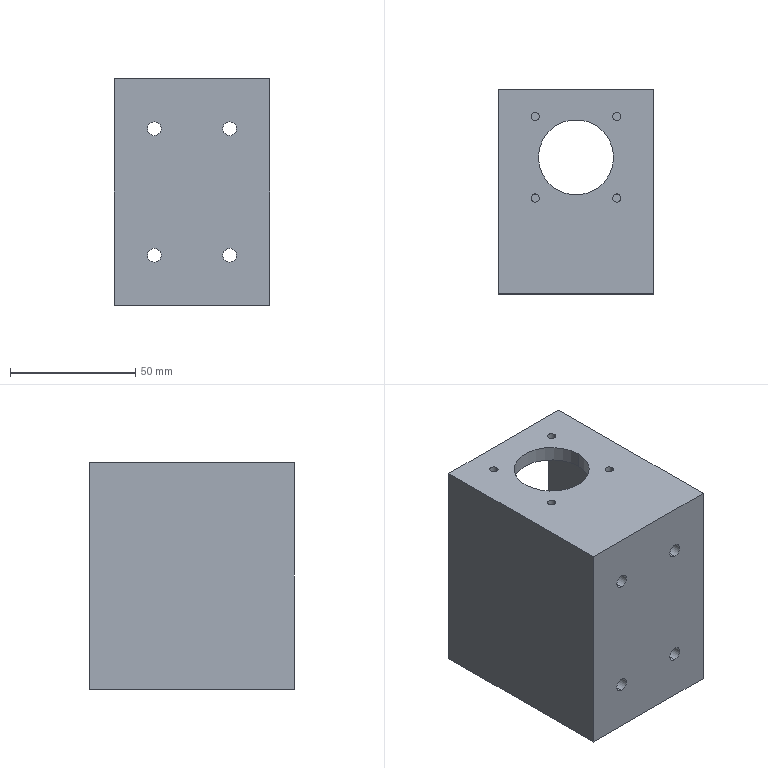Part | Creo | features CURVE 7, CUT 4, DATUM PLANE 3, PROTRUSION 2, CHAMFER 1, COORDINATE SYSTEM 1 | 1 solid | 45 faces | box 62 x 81.5 x 90.5 mm | volume 211765 mm3 | cylinder 26 | plane 19 | commonest cylinder face diameters 3.3 x8 5.5 x8 4.2 x6 30 x2 34 x2
STEP:
#1=CARTESIAN_POINT('',(0.,0.,0.));
#2=DIRECTION('',(0.,0.,1.));
#3=DIRECTION('',(1.,0.,0.));
#4=AXIS2_PLACEMENT_3D('',#1,#2,#3);
#5=CARTESIAN_POINT('',(31.,27.,0.));
#6=VERTEX_POINT('',#5);
#7=CARTESIAN_POINT('',(-31.,27.,0.));
#8=VERTEX_POINT('',#7);
#9=CARTESIAN_POINT('',(31.,27.,0.));
#10=DIRECTION('',(-1.,0.,0.));
#11=VECTOR('',#10,62.);
#12=LINE('',#9,#11);
#13=EDGE_CURVE('',#6,#8,#12,.T.);
#14=ORIENTED_EDGE('',*,*,#13,.T.);
#15=CARTESIAN_POINT('',(-31.,-54.5,0.));
#16=VERTEX_POINT('',#15);
#17=CARTESIAN_POINT('',(-31.,27.,0.));
#18=DIRECTION('',(0.,-1.,0.));
#19=VECTOR('',#18,81.5);
#20=LINE('',#17,#19);
#21=EDGE_CURVE('',#8,#16,#20,.T.);
#22=ORIENTED_EDGE('',*,*,#21,.T.);
#23=CARTESIAN_POINT('',(31.,-54.5,0.));
#24=VERTEX_POINT('',#23);
#25=CARTESIAN_POINT('',(-31.,-54.5,0.));
#26=DIRECTION('',(1.,0.,0.));
#27=VECTOR('',#26,62.);
#28=LINE('',#25,#27);
#29=EDGE_CURVE('',#16,#24,#28,.T.);
#30=ORIENTED_EDGE('',*,*,#29,.T.);
#31=CARTESIAN_POINT('',(31.,-54.5,0.));
#32=DIRECTION('',(0.,1.,0.));
#33=VECTOR('',#32,81.5);
#34=LINE('',#31,#33);
#35=EDGE_CURVE('',#24,#6,#34,.T.);
#36=ORIENTED_EDGE('',*,*,#35,.T.);
#37=EDGE_LOOP('',(#14,#22,#30,#36));
#38=FACE_OUTER_BOUND('',#37,.F.);
#39=CARTESIAN_POINT('',(0.,-17.,0.));
#40=VERTEX_POINT('',#39);
#41=CARTESIAN_POINT('',(0.,17.,0.));
#42=VERTEX_POINT('',#41);
#43=CARTESIAN_POINT('',(0.,0.,0.));
#44=DIRECTION('',(0.,0.,-1.));
#45=DIRECTION('',(0.,-1.,0.));
#46=AXIS2_PLACEMENT_3D('',#43,#44,#45);
#47=CIRCLE('',#46,17.);
#48=EDGE_CURVE('',#40,#42,#47,.T.);
#49=ORIENTED_EDGE('',*,*,#48,.T.);
#50=CARTESIAN_POINT('',(0.,0.,0.));
#51=DIRECTION('',(0.,0.,-1.));
#52=DIRECTION('',(0.,1.,0.));
#53=AXIS2_PLACEMENT_3D('',#50,#51,#52);
#54=CIRCLE('',#53,17.);
#55=EDGE_CURVE('',#42,#40,#54,.T.);
#56=ORIENTED_EDGE('',*,*,#55,.T.);
#57=EDGE_LOOP('',(#49,#56));
#58=FACE_BOUND('',#57,.F.);
#59=CARTESIAN_POINT('',(0.,18.9,0.));
#60=VERTEX_POINT('',#59);
#61=CARTESIAN_POINT('',(0.,23.1,0.));
#62=VERTEX_POINT('',#61);
#63=CARTESIAN_POINT('',(0.,21.,0.));
#64=DIRECTION('',(0.,0.,-1.));
#65=DIRECTION('',(0.,-1.,0.));
#66=AXIS2_PLACEMENT_3D('',#63,#64,#65);
#67=CIRCLE('',#66,2.1);
#68=EDGE_CURVE('',#60,#62,#67,.T.);
#69=ORIENTED_EDGE('',*,*,#68,.T.);
#70=CARTESIAN_POINT('',(0.,21.,0.));
#71=DIRECTION('',(0.,0.,-1.));
#72=DIRECTION('',(0.,1.,0.));
#73=AXIS2_PLACEMENT_3D('',#70,#71,#72);
#74=CIRCLE('',#73,2.1);
#75=EDGE_CURVE('',#62,#60,#74,.T.);
#76=ORIENTED_EDGE('',*,*,#75,.T.);
#77=EDGE_LOOP('',(#69,#76));
#78=FACE_BOUND('',#77,.F.);
#79=CARTESIAN_POINT('',(-18.187,-12.6,0.));
#80=VERTEX_POINT('',#79);
#81=CARTESIAN_POINT('',(-18.187,-8.4,0.));
#82=VERTEX_POINT('',#81);
#83=CARTESIAN_POINT('',(-18.187,-10.5,0.));
#84=DIRECTION('',(0.,0.,-1.));
#85=DIRECTION('',(0.,-1.,0.));
#86=AXIS2_PLACEMENT_3D('',#83,#84,#85);
#87=CIRCLE('',#86,2.1);
#88=EDGE_CURVE('',#80,#82,#87,.T.);
#89=ORIENTED_EDGE('',*,*,#88,.T.);
#90=CARTESIAN_POINT('',(-18.187,-10.5,0.));
#91=DIRECTION('',(0.,0.,-1.));
#92=DIRECTION('',(0.,1.,0.));
#93=AXIS2_PLACEMENT_3D('',#90,#91,#92);
#94=CIRCLE('',#93,2.1);
#95=EDGE_CURVE('',#82,#80,#94,.T.);
#96=ORIENTED_EDGE('',*,*,#95,.T.);
#97=EDGE_LOOP('',(#89,#96));
#98=FACE_BOUND('',#97,.F.);
#99=CARTESIAN_POINT('',(18.187,-12.6,0.));
#100=VERTEX_POINT('',#99);
#101=CARTESIAN_POINT('',(18.187,-8.4,0.));
#102=VERTEX_POINT('',#101);
#103=CARTESIAN_POINT('',(18.187,-10.5,0.));
#104=DIRECTION('',(0.,0.,-1.));
#105=DIRECTION('',(0.,-1.,0.));
#106=AXIS2_PLACEMENT_3D('',#103,#104,#105);
#107=CIRCLE('',#106,2.1);
#108=EDGE_CURVE('',#100,#102,#107,.T.);
#109=ORIENTED_EDGE('',*,*,#108,.T.);
#110=CARTESIAN_POINT('',(18.187,-10.5,0.));
#111=DIRECTION('',(0.,0.,-1.));
#112=DIRECTION('',(0.,1.,0.));
#113=AXIS2_PLACEMENT_3D('',#110,#111,#112);
#114=CIRCLE('',#113,2.1);
#115=EDGE_CURVE('',#102,#100,#114,.T.);
#116=ORIENTED_EDGE('',*,*,#115,.T.);
#117=EDGE_LOOP('',(#109,#116));
#118=FACE_BOUND('',#117,.F.);
#119=CARTESIAN_POINT('',(0.,0.,0.));
#120=DIRECTION('',(0.,0.,1.));
#121=DIRECTION('',(1.,0.,0.));
#122=AXIS2_PLACEMENT_3D('',#119,#120,#121);
#123=PLANE('',#122);
#124=ADVANCED_FACE('',(#38,#58,#78,#98,#118),#123,.F.);
#125=ORIENTED_EDGE('',*,*,#13,.F.);
#126=CARTESIAN_POINT('',(31.,27.,90.5));
#127=VERTEX_POINT('',#126);
#128=CARTESIAN_POINT('',(31.,27.,0.));
#129=DIRECTION('',(0.,0.,1.));
#130=VECTOR('',#129,90.5);
#131=LINE('',#128,#130);
#132=EDGE_CURVE('',#6,#127,#131,.T.);
#133=ORIENTED_EDGE('',*,*,#132,.T.);
#134=CARTESIAN_POINT('',(-31.,27.,90.5));
#135=VERTEX_POINT('',#134);
#136=CARTESIAN_POINT('',(31.,27.,90.5));
#137=DIRECTION('',(-1.,0.,0.));
#138=VECTOR('',#137,62.);
#139=LINE('',#136,#138);
#140=EDGE_CURVE('',#127,#135,#139,.T.);
#141=ORIENTED_EDGE('',*,*,#140,.T.);
#142=CARTESIAN_POINT('',(-31.,27.,0.));
#143=DIRECTION('',(0.,0.,1.));
#144=VECTOR('',#143,90.5);
#145=LINE('',#142,#144);
#146=EDGE_CURVE('',#8,#135,#145,.T.);
#147=ORIENTED_EDGE('',*,*,#146,.F.);
#148=EDGE_LOOP('',(#125,#133,#141,#147));
#149=FACE_OUTER_BOUND('',#148,.F.);
#150=CARTESIAN_POINT('',(-25.,27.,9.));
#151=VERTEX_POINT('',#150);
#152=CARTESIAN_POINT('',(-25.,27.,81.5));
#153=VERTEX_POINT('',#152);
#154=CARTESIAN_POINT('',(-25.,27.,9.));
#155=DIRECTION('',(0.,0.,1.));
#156=VECTOR('',#155,72.5);
#157=LINE('',#154,#156);
#158=EDGE_CURVE('',#151,#153,#157,.T.);
#159=ORIENTED_EDGE('',*,*,#158,.T.);
#160=CARTESIAN_POINT('',(-22.,27.,84.5));
#161=VERTEX_POINT('',#160);
#162=CARTESIAN_POINT('',(-22.,27.,84.5));
#163=DIRECTION('',(-0.7071,0.,-0.7071));
#164=VECTOR('',#163,4.243);
#165=LINE('',#162,#164);
#166=EDGE_CURVE('',#161,#153,#165,.T.);
#167=ORIENTED_EDGE('',*,*,#166,.F.);
#168=CARTESIAN_POINT('',(22.,27.,84.5));
#169=VERTEX_POINT('',#168);
#170=CARTESIAN_POINT('',(-22.,27.,84.5));
#171=DIRECTION('',(1.,0.,0.));
#172=VECTOR('',#171,44.);
#173=LINE('',#170,#172);
#174=EDGE_CURVE('',#161,#169,#173,.T.);
#175=ORIENTED_EDGE('',*,*,#174,.T.);
#176=CARTESIAN_POINT('',(25.,27.,81.5));
#177=VERTEX_POINT('',#176);
#178=CARTESIAN_POINT('',(25.,27.,81.5));
#179=DIRECTION('',(-0.7071,0.,0.7071));
#180=VECTOR('',#179,4.243);
#181=LINE('',#178,#180);
#182=EDGE_CURVE('',#177,#169,#181,.T.);
#183=ORIENTED_EDGE('',*,*,#182,.F.);
#184=CARTESIAN_POINT('',(25.,27.,9.));
#185=VERTEX_POINT('',#184);
#186=CARTESIAN_POINT('',(25.,27.,81.5));
#187=DIRECTION('',(0.,0.,-1.));
#188=VECTOR('',#187,72.5);
#189=LINE('',#186,#188);
#190=EDGE_CURVE('',#177,#185,#189,.T.);
#191=ORIENTED_EDGE('',*,*,#190,.T.);
#192=CARTESIAN_POINT('',(22.,27.,6.));
#193=VERTEX_POINT('',#192);
#194=CARTESIAN_POINT('',(22.,27.,6.));
#195=DIRECTION('',(0.7071,0.,0.7071));
#196=VECTOR('',#195,4.243);
#197=LINE('',#194,#196);
#198=EDGE_CURVE('',#193,#185,#197,.T.);
#199=ORIENTED_EDGE('',*,*,#198,.F.);
#200=CARTESIAN_POINT('',(-22.,27.,6.));
#201=VERTEX_POINT('',#200);
#202=CARTESIAN_POINT('',(22.,27.,6.));
#203=DIRECTION('',(-1.,0.,0.));
#204=VECTOR('',#203,44.);
#205=LINE('',#202,#204);
#206=EDGE_CURVE('',#193,#201,#205,.T.);
#207=ORIENTED_EDGE('',*,*,#206,.T.);
#208=CARTESIAN_POINT('',(-25.,27.,9.));
#209=DIRECTION('',(0.7071,0.,-0.7071));
#210=VECTOR('',#209,4.243);
#211=LINE('',#208,#210);
#212=EDGE_CURVE('',#151,#201,#211,.T.);
#213=ORIENTED_EDGE('',*,*,#212,.F.);
#214=EDGE_LOOP('',(#159,#167,#175,#183,#191,#199,#207,#213));
#215=FACE_BOUND('',#214,.F.);
#216=CARTESIAN_POINT('',(31.,27.,0.));
#217=DIRECTION('',(0.,1.,0.));
#218=DIRECTION('',(-1.,0.,0.));
#219=AXIS2_PLACEMENT_3D('',#216,#217,#218);
#220=PLANE('',#219);
#221=ADVANCED_FACE('',(#149,#215),#220,.T.);
#222=ORIENTED_EDGE('',*,*,#35,.F.);
#223=CARTESIAN_POINT('',(31.,-54.5,90.5));
#224=VERTEX_POINT('',#223);
#225=CARTESIAN_POINT('',(31.,-54.5,0.));
#226=DIRECTION('',(0.,0.,1.));
#227=VECTOR('',#226,90.5);
#228=LINE('',#225,#227);
#229=EDGE_CURVE('',#24,#224,#228,.T.);
#230=ORIENTED_EDGE('',*,*,#229,.T.);
#231=CARTESIAN_POINT('',(31.,-54.5,90.5));
#232=DIRECTION('',(0.,1.,0.));
#233=VECTOR('',#232,81.5);
#234=LINE('',#231,#233);
#235=EDGE_CURVE('',#224,#127,#234,.T.);
#236=ORIENTED_EDGE('',*,*,#235,.T.);
#237=ORIENTED_EDGE('',*,*,#132,.F.);
#238=EDGE_LOOP('',(#222,#230,#236,#237));
#239=FACE_OUTER_BOUND('',#238,.F.);
#240=CARTESIAN_POINT('',(31.,-54.5,0.));
#241=DIRECTION('',(1.,0.,0.));
#242=DIRECTION('',(0.,1.,0.));
#243=AXIS2_PLACEMENT_3D('',#240,#241,#242);
#244=PLANE('',#243);
#245=ADVANCED_FACE('',(#239),#244,.T.);
#246=ORIENTED_EDGE('',*,*,#29,.F.);
#247=CARTESIAN_POINT('',(-31.,-54.5,90.5));
#248=VERTEX_POINT('',#247);
#249=CARTESIAN_POINT('',(-31.,-54.5,0.));
#250=DIRECTION('',(0.,0.,1.));
#251=VECTOR('',#250,90.5);
#252=LINE('',#249,#251);
#253=EDGE_CURVE('',#16,#248,#252,.T.);
#254=ORIENTED_EDGE('',*,*,#253,.T.);
#255=CARTESIAN_POINT('',(-31.,-54.5,90.5));
#256=DIRECTION('',(1.,0.,0.));
#257=VECTOR('',#256,62.);
#258=LINE('',#255,#257);
#259=EDGE_CURVE('',#248,#224,#258,.T.);
#260=ORIENTED_EDGE('',*,*,#259,.T.);
#261=ORIENTED_EDGE('',*,*,#229,.F.);
#262=EDGE_LOOP('',(#246,#254,#260,#261));
#263=FACE_OUTER_BOUND('',#262,.F.);
#264=CARTESIAN_POINT('',(-15.,-54.5,67.75));
#265=VERTEX_POINT('',#264);
#266=CARTESIAN_POINT('',(-15.,-54.5,73.25));
#267=VERTEX_POINT('',#266);
#268=CARTESIAN_POINT('',(-15.,-54.5,70.5));
#269=DIRECTION('',(0.,1.,0.));
#270=DIRECTION('',(0.,0.,-1.));
#271=AXIS2_PLACEMENT_3D('',#268,#269,#270);
#272=CIRCLE('',#271,2.75);
#273=EDGE_CURVE('',#265,#267,#272,.T.);
#274=ORIENTED_EDGE('',*,*,#273,.F.);
#275=CARTESIAN_POINT('',(-15.,-54.5,70.5));
#276=DIRECTION('',(0.,1.,0.));
#277=DIRECTION('',(0.,0.,1.));
#278=AXIS2_PLACEMENT_3D('',#275,#276,#277);
#279=CIRCLE('',#278,2.75);
#280=EDGE_CURVE('',#267,#265,#279,.T.);
#281=ORIENTED_EDGE('',*,*,#280,.F.);
#282=EDGE_LOOP('',(#274,#281));
#283=FACE_BOUND('',#282,.F.);
#284=CARTESIAN_POINT('',(-15.,-54.5,17.25));
#285=VERTEX_POINT('',#284);
#286=CARTESIAN_POINT('',(-15.,-54.5,22.75));
#287=VERTEX_POINT('',#286);
#288=CARTESIAN_POINT('',(-15.,-54.5,20.));
#289=DIRECTION('',(0.,1.,0.));
#290=DIRECTION('',(0.,0.,-1.));
#291=AXIS2_PLACEMENT_3D('',#288,#289,#290);
#292=CIRCLE('',#291,2.75);
#293=EDGE_CURVE('',#285,#287,#292,.T.);
#294=ORIENTED_EDGE('',*,*,#293,.F.);
#295=CARTESIAN_POINT('',(-15.,-54.5,20.));
#296=DIRECTION('',(0.,1.,0.));
#297=DIRECTION('',(0.,0.,1.));
#298=AXIS2_PLACEMENT_3D('',#295,#296,#297);
#299=CIRCLE('',#298,2.75);
#300=EDGE_CURVE('',#287,#285,#299,.T.);
#301=ORIENTED_EDGE('',*,*,#300,.F.);
#302=EDGE_LOOP('',(#294,#301));
#303=FACE_BOUND('',#302,.F.);
#304=CARTESIAN_POINT('',(15.,-54.5,17.25));
#305=VERTEX_POINT('',#304);
#306=CARTESIAN_POINT('',(15.,-54.5,22.75));
#307=VERTEX_POINT('',#306);
#308=CARTESIAN_POINT('',(15.,-54.5,20.));
#309=DIRECTION('',(0.,1.,0.));
#310=DIRECTION('',(0.,0.,-1.));
#311=AXIS2_PLACEMENT_3D('',#308,#309,#310);
#312=CIRCLE('',#311,2.75);
#313=EDGE_CURVE('',#305,#307,#312,.T.);
#314=ORIENTED_EDGE('',*,*,#313,.F.);
#315=CARTESIAN_POINT('',(15.,-54.5,20.));
#316=DIRECTION('',(0.,1.,0.));
#317=DIRECTION('',(0.,0.,1.));
#318=AXIS2_PLACEMENT_3D('',#315,#316,#317);
#319=CIRCLE('',#318,2.75);
#320=EDGE_CURVE('',#307,#305,#319,.T.);
#321=ORIENTED_EDGE('',*,*,#320,.F.);
#322=EDGE_LOOP('',(#314,#321));
#323=FACE_BOUND('',#322,.F.);
#324=CARTESIAN_POINT('',(15.,-54.5,67.75));
#325=VERTEX_POINT('',#324);
#326=CARTESIAN_POINT('',(15.,-54.5,73.25));
#327=VERTEX_POINT('',#326);
#328=CARTESIAN_POINT('',(15.,-54.5,70.5));
#329=DIRECTION('',(0.,1.,0.));
#330=DIRECTION('',(0.,0.,-1.));
#331=AXIS2_PLACEMENT_3D('',#328,#329,#330);
#332=CIRCLE('',#331,2.75);
#333=EDGE_CURVE('',#325,#327,#332,.T.);
#334=ORIENTED_EDGE('',*,*,#333,.F.);
#335=CARTESIAN_POINT('',(15.,-54.5,70.5));
#336=DIRECTION('',(0.,1.,0.));
#337=DIRECTION('',(0.,0.,1.));
#338=AXIS2_PLACEMENT_3D('',#335,#336,#337);
#339=CIRCLE('',#338,2.75);
#340=EDGE_CURVE('',#327,#325,#339,.T.);
#341=ORIENTED_EDGE('',*,*,#340,.F.);
#342=EDGE_LOOP('',(#334,#341));
#343=FACE_BOUND('',#342,.F.);
#344=CARTESIAN_POINT('',(-31.,-54.5,0.));
#345=DIRECTION('',(0.,-1.,0.));
#346=DIRECTION('',(1.,0.,0.));
#347=AXIS2_PLACEMENT_3D('',#344,#345,#346);
#348=PLANE('',#347);
#349=ADVANCED_FACE('',(#263,#283,#303,#323,#343),#348,.T.);
#350=ORIENTED_EDGE('',*,*,#21,.F.);
#351=ORIENTED_EDGE('',*,*,#146,.T.);
#352=CARTESIAN_POINT('',(-31.,27.,90.5));
#353=DIRECTION('',(0.,-1.,0.));
#354=VECTOR('',#353,81.5);
#355=LINE('',#352,#354);
#356=EDGE_CURVE('',#135,#248,#355,.T.);
#357=ORIENTED_EDGE('',*,*,#356,.T.);
#358=ORIENTED_EDGE('',*,*,#253,.F.);
#359=EDGE_LOOP('',(#350,#351,#357,#358));
#360=FACE_OUTER_BOUND('',#359,.F.);
#361=CARTESIAN_POINT('',(-31.,27.,0.));
#362=DIRECTION('',(-1.,0.,0.));
#363=DIRECTION('',(0.,-1.,0.));
#364=AXIS2_PLACEMENT_3D('',#361,#362,#363);
#365=PLANE('',#364);
#366=ADVANCED_FACE('',(#360),#365,.T.);
#367=ORIENTED_EDGE('',*,*,#140,.F.);
#368=ORIENTED_EDGE('',*,*,#235,.F.);
#369=ORIENTED_EDGE('',*,*,#259,.F.);
#370=ORIENTED_EDGE('',*,*,#356,.F.);
#371=EDGE_LOOP('',(#367,#368,#369,#370));
#372=FACE_OUTER_BOUND('',#371,.F.);
#373=CARTESIAN_POINT('',(-14.61,16.26,90.5));
#374=VERTEX_POINT('',#373);
#375=CARTESIAN_POINT('',(-17.91,16.26,90.5));
#376=VERTEX_POINT('',#375);
#377=CARTESIAN_POINT('',(-16.26,16.26,90.5));
#378=DIRECTION('',(0.,0.,-1.));
#379=DIRECTION('',(1.,0.,0.));
#380=AXIS2_PLACEMENT_3D('',#377,#378,#379);
#381=CIRCLE('',#380,1.65);
#382=EDGE_CURVE('',#374,#376,#381,.T.);
#383=ORIENTED_EDGE('',*,*,#382,.F.);
#384=CARTESIAN_POINT('',(-16.26,16.26,90.5));
#385=DIRECTION('',(0.,0.,-1.));
#386=DIRECTION('',(-1.,0.,0.));
#387=AXIS2_PLACEMENT_3D('',#384,#385,#386);
#388=CIRCLE('',#387,1.65);
#389=EDGE_CURVE('',#376,#374,#388,.T.);
#390=ORIENTED_EDGE('',*,*,#389,.F.);
#391=EDGE_LOOP('',(#383,#390));
#392=FACE_BOUND('',#391,.F.);
#393=CARTESIAN_POINT('',(17.91,16.26,90.5));
#394=VERTEX_POINT('',#393);
#395=CARTESIAN_POINT('',(14.61,16.26,90.5));
#396=VERTEX_POINT('',#395);
#397=CARTESIAN_POINT('',(16.26,16.26,90.5));
#398=DIRECTION('',(0.,0.,-1.));
#399=DIRECTION('',(1.,0.,0.));
#400=AXIS2_PLACEMENT_3D('',#397,#398,#399);
#401=CIRCLE('',#400,1.65);
#402=EDGE_CURVE('',#394,#396,#401,.T.);
#403=ORIENTED_EDGE('',*,*,#402,.F.);
#404=CARTESIAN_POINT('',(16.26,16.26,90.5));
#405=DIRECTION('',(0.,0.,-1.));
#406=DIRECTION('',(-1.,0.,0.));
#407=AXIS2_PLACEMENT_3D('',#404,#405,#406);
#408=CIRCLE('',#407,1.65);
#409=EDGE_CURVE('',#396,#394,#408,.T.);
#410=ORIENTED_EDGE('',*,*,#409,.F.);
#411=EDGE_LOOP('',(#403,#410));
#412=FACE_BOUND('',#411,.F.);
#413=CARTESIAN_POINT('',(17.91,-16.26,90.5));
#414=VERTEX_POINT('',#413);
#415=CARTESIAN_POINT('',(14.61,-16.26,90.5));
#416=VERTEX_POINT('',#415);
#417=CARTESIAN_POINT('',(16.26,-16.26,90.5));
#418=DIRECTION('',(0.,0.,-1.));
#419=DIRECTION('',(1.,0.,0.));
#420=AXIS2_PLACEMENT_3D('',#417,#418,#419);
#421=CIRCLE('',#420,1.65);
#422=EDGE_CURVE('',#414,#416,#421,.T.);
#423=ORIENTED_EDGE('',*,*,#422,.F.);
#424=CARTESIAN_POINT('',(16.26,-16.26,90.5));
#425=DIRECTION('',(0.,0.,-1.));
#426=DIRECTION('',(-1.,0.,0.));
#427=AXIS2_PLACEMENT_3D('',#424,#425,#426);
#428=CIRCLE('',#427,1.65);
#429=EDGE_CURVE('',#416,#414,#428,.T.);
#430=ORIENTED_EDGE('',*,*,#429,.F.);
#431=EDGE_LOOP('',(#423,#430));
#432=FACE_BOUND('',#431,.F.);
#433=CARTESIAN_POINT('',(-14.61,-16.26,90.5));
#434=VERTEX_POINT('',#433);
#435=CARTESIAN_POINT('',(-17.91,-16.26,90.5));
#436=VERTEX_POINT('',#435);
#437=CARTESIAN_POINT('',(-16.26,-16.26,90.5));
#438=DIRECTION('',(0.,0.,-1.));
#439=DIRECTION('',(1.,0.,0.));
#440=AXIS2_PLACEMENT_3D('',#437,#438,#439);
#441=CIRCLE('',#440,1.65);
#442=EDGE_CURVE('',#434,#436,#441,.T.);
#443=ORIENTED_EDGE('',*,*,#442,.F.);
#444=CARTESIAN_POINT('',(-16.26,-16.26,90.5));
#445=DIRECTION('',(0.,0.,-1.));
#446=DIRECTION('',(-1.,0.,0.));
#447=AXIS2_PLACEMENT_3D('',#444,#445,#446);
#448=CIRCLE('',#447,1.65);
#449=EDGE_CURVE('',#436,#434,#448,.T.);
#450=ORIENTED_EDGE('',*,*,#449,.F.);
#451=EDGE_LOOP('',(#443,#450));
#452=FACE_BOUND('',#451,.F.);
#453=CARTESIAN_POINT('',(15.,0.,90.5));
#454=VERTEX_POINT('',#453);
#455=CARTESIAN_POINT('',(-15.,0.,90.5));
#456=VERTEX_POINT('',#455);
#457=CARTESIAN_POINT('',(0.,0.,90.5));
#458=DIRECTION('',(0.,0.,-1.));
#459=DIRECTION('',(1.,0.,0.));
#460=AXIS2_PLACEMENT_3D('',#457,#458,#459);
#461=CIRCLE('',#460,15.);
#462=EDGE_CURVE('',#454,#456,#461,.T.);
#463=ORIENTED_EDGE('',*,*,#462,.F.);
#464=CARTESIAN_POINT('',(0.,0.,90.5));
#465=DIRECTION('',(0.,0.,-1.));
#466=DIRECTION('',(-1.,0.,0.));
#467=AXIS2_PLACEMENT_3D('',#464,#465,#466);
#468=CIRCLE('',#467,15.);
#469=EDGE_CURVE('',#456,#454,#468,.T.);
#470=ORIENTED_EDGE('',*,*,#469,.F.);
#471=EDGE_LOOP('',(#463,#470));
#472=FACE_BOUND('',#471,.F.);
#473=CARTESIAN_POINT('',(0.,0.,90.5));
#474=DIRECTION('',(0.,0.,1.));
#475=DIRECTION('',(1.,0.,0.));
#476=AXIS2_PLACEMENT_3D('',#473,#474,#475);
#477=PLANE('',#476);
#478=ADVANCED_FACE('',(#372,#392,#412,#432,#452,#472),#477,.T.);
#479=CARTESIAN_POINT('',(-15.,0.,84.5));
#480=VERTEX_POINT('',#479);
#481=CARTESIAN_POINT('',(15.,0.,84.5));
#482=VERTEX_POINT('',#481);
#483=CARTESIAN_POINT('',(0.,0.,84.5));
#484=DIRECTION('',(0.,0.,1.));
#485=DIRECTION('',(-1.,0.,0.));
#486=AXIS2_PLACEMENT_3D('',#483,#484,#485);
#487=CIRCLE('',#486,15.);
#488=EDGE_CURVE('',#480,#482,#487,.T.);
#489=ORIENTED_EDGE('',*,*,#488,.T.);
#490=CARTESIAN_POINT('',(15.,0.,84.5));
#491=DIRECTION('',(0.,0.,1.));
#492=VECTOR('',#491,6.);
#493=LINE('',#490,#492);
#494=EDGE_CURVE('',#482,#454,#493,.T.);
#495=ORIENTED_EDGE('',*,*,#494,.T.);
#496=ORIENTED_EDGE('',*,*,#462,.T.);
#497=CARTESIAN_POINT('',(-15.,0.,84.5));
#498=DIRECTION('',(0.,0.,1.));
#499=VECTOR('',#498,6.);
#500=LINE('',#497,#499);
#501=EDGE_CURVE('',#480,#456,#500,.T.);
#502=ORIENTED_EDGE('',*,*,#501,.F.);
#503=EDGE_LOOP('',(#489,#495,#496,#502));
#504=FACE_OUTER_BOUND('',#503,.F.);
#505=CARTESIAN_POINT('',(0.,0.,0.));
#506=DIRECTION('',(0.,0.,1.));
#507=DIRECTION('',(1.,0.,0.));
#508=AXIS2_PLACEMENT_3D('',#505,#506,#507);
#509=CYLINDRICAL_SURFACE('',#508,15.);
#510=ADVANCED_FACE('',(#504),#509,.F.);
#511=CARTESIAN_POINT('',(22.,-30.,84.5));
#512=VERTEX_POINT('',#511);
#513=CARTESIAN_POINT('',(22.,27.,84.5));
#514=DIRECTION('',(0.,-1.,0.));
#515=VECTOR('',#514,57.);
#516=LINE('',#513,#515);
#517=EDGE_CURVE('',#169,#512,#516,.T.);
#518=ORIENTED_EDGE('',*,*,#517,.F.);
#519=ORIENTED_EDGE('',*,*,#174,.F.);
#520=CARTESIAN_POINT('',(-22.,-30.,84.5));
#521=VERTEX_POINT('',#520);
#522=CARTESIAN_POINT('',(-22.,27.,84.5));
#523=DIRECTION('',(0.,-1.,0.));
#524=VECTOR('',#523,57.);
#525=LINE('',#522,#524);
#526=EDGE_CURVE('',#161,#521,#525,.T.);
#527=ORIENTED_EDGE('',*,*,#526,.T.);
#528=CARTESIAN_POINT('',(22.,-30.,84.5));
#529=DIRECTION('',(-1.,0.,0.));
#530=VECTOR('',#529,44.);
#531=LINE('',#528,#530);
#532=EDGE_CURVE('',#512,#521,#531,.T.);
#533=ORIENTED_EDGE('',*,*,#532,.F.);
#534=EDGE_LOOP('',(#518,#519,#527,#533));
#535=FACE_OUTER_BOUND('',#534,.F.);
#536=CARTESIAN_POINT('',(-17.91,16.26,84.5));
#537=VERTEX_POINT('',#536);
#538=CARTESIAN_POINT('',(-14.61,16.26,84.5));
#539=VERTEX_POINT('',#538);
#540=CARTESIAN_POINT('',(-16.26,16.26,84.5));
#541=DIRECTION('',(0.,0.,1.));
#542=DIRECTION('',(-1.,0.,0.));
#543=AXIS2_PLACEMENT_3D('',#540,#541,#542);
#544=CIRCLE('',#543,1.65);
#545=EDGE_CURVE('',#537,#539,#544,.T.);
#546=ORIENTED_EDGE('',*,*,#545,.F.);
#547=CARTESIAN_POINT('',(-16.26,16.26,84.5));
#548=DIRECTION('',(0.,0.,1.));
#549=DIRECTION('',(1.,0.,0.));
#550=AXIS2_PLACEMENT_3D('',#547,#548,#549);
#551=CIRCLE('',#550,1.65);
#552=EDGE_CURVE('',#539,#537,#551,.T.);
#553=ORIENTED_EDGE('',*,*,#552,.F.);
#554=EDGE_LOOP('',(#546,#553));
#555=FACE_BOUND('',#554,.F.);
#556=CARTESIAN_POINT('',(14.61,16.26,84.5));
#557=VERTEX_POINT('',#556);
#558=CARTESIAN_POINT('',(17.91,16.26,84.5));
#559=VERTEX_POINT('',#558);
#560=CARTESIAN_POINT('',(16.26,16.26,84.5));
#561=DIRECTION('',(0.,0.,1.));
#562=DIRECTION('',(-1.,0.,0.));
#563=AXIS2_PLACEMENT_3D('',#560,#561,#562);
#564=CIRCLE('',#563,1.65);
#565=EDGE_CURVE('',#557,#559,#564,.T.);
#566=ORIENTED_EDGE('',*,*,#565,.F.);
#567=CARTESIAN_POINT('',(16.26,16.26,84.5));
#568=DIRECTION('',(0.,0.,1.));
#569=DIRECTION('',(1.,0.,0.));
#570=AXIS2_PLACEMENT_3D('',#567,#568,#569);
#571=CIRCLE('',#570,1.65);
#572=EDGE_CURVE('',#559,#557,#571,.T.);
#573=ORIENTED_EDGE('',*,*,#572,.F.);
#574=EDGE_LOOP('',(#566,#573));
#575=FACE_BOUND('',#574,.F.);
#576=CARTESIAN_POINT('',(14.61,-16.26,84.5));
#577=VERTEX_POINT('',#576);
#578=CARTESIAN_POINT('',(17.91,-16.26,84.5));
#579=VERTEX_POINT('',#578);
#580=CARTESIAN_POINT('',(16.26,-16.26,84.5));
#581=DIRECTION('',(0.,0.,1.));
#582=DIRECTION('',(-1.,0.,0.));
#583=AXIS2_PLACEMENT_3D('',#580,#581,#582);
#584=CIRCLE('',#583,1.65);
#585=EDGE_CURVE('',#577,#579,#584,.T.);
#586=ORIENTED_EDGE('',*,*,#585,.F.);
#587=CARTESIAN_POINT('',(16.26,-16.26,84.5));
#588=DIRECTION('',(0.,0.,1.));
#589=DIRECTION('',(1.,0.,0.));
#590=AXIS2_PLACEMENT_3D('',#587,#588,#589);
#591=CIRCLE('',#590,1.65);
#592=EDGE_CURVE('',#579,#577,#591,.T.);
#593=ORIENTED_EDGE('',*,*,#592,.F.);
#594=EDGE_LOOP('',(#586,#593));
#595=FACE_BOUND('',#594,.F.);
#596=CARTESIAN_POINT('',(-17.91,-16.26,84.5));
#597=VERTEX_POINT('',#596);
#598=CARTESIAN_POINT('',(-14.61,-16.26,84.5));
#599=VERTEX_POINT('',#598);
#600=CARTESIAN_POINT('',(-16.26,-16.26,84.5));
#601=DIRECTION('',(0.,0.,1.));
#602=DIRECTION('',(-1.,0.,0.));
#603=AXIS2_PLACEMENT_3D('',#600,#601,#602);
#604=CIRCLE('',#603,1.65);
#605=EDGE_CURVE('',#597,#599,#604,.T.);
#606=ORIENTED_EDGE('',*,*,#605,.F.);
#607=CARTESIAN_POINT('',(-16.26,-16.26,84.5));
#608=DIRECTION('',(0.,0.,1.));
#609=DIRECTION('',(1.,0.,0.));
#610=AXIS2_PLACEMENT_3D('',#607,#608,#609);
#611=CIRCLE('',#610,1.65);
#612=EDGE_CURVE('',#599,#597,#611,.T.);
#613=ORIENTED_EDGE('',*,*,#612,.F.);
#614=EDGE_LOOP('',(#606,#613));
#615=FACE_BOUND('',#614,.F.);
#616=ORIENTED_EDGE('',*,*,#488,.F.);
#617=CARTESIAN_POINT('',(0.,0.,84.5));
#618=DIRECTION('',(0.,0.,1.));
#619=DIRECTION('',(1.,0.,0.));
#620=AXIS2_PLACEMENT_3D('',#617,#618,#619);
#621=CIRCLE('',#620,15.);
#622=EDGE_CURVE('',#482,#480,#621,.T.);
#623=ORIENTED_EDGE('',*,*,#622,.F.);
#624=EDGE_LOOP('',(#616,#623));
#625=FACE_BOUND('',#624,.F.);
#626=CARTESIAN_POINT('',(-25.,27.,84.5));
#627=DIRECTION('',(0.,0.,1.));
#628=DIRECTION('',(1.,0.,0.));
#629=AXIS2_PLACEMENT_3D('',#626,#627,#628);
#630=PLANE('',#629);
#631=ADVANCED_FACE('',(#535,#555,#575,#595,#615,#625),#630,.F.);
#632=ORIENTED_EDGE('',*,*,#622,.T.);
#633=ORIENTED_EDGE('',*,*,#501,.T.);
#634=ORIENTED_EDGE('',*,*,#469,.T.);
#635=ORIENTED_EDGE('',*,*,#494,.F.);
#636=EDGE_LOOP('',(#632,#633,#634,#635));
#637=FACE_OUTER_BOUND('',#636,.F.);
#638=CARTESIAN_POINT('',(0.,0.,0.));
#639=DIRECTION('',(0.,0.,1.));
#640=DIRECTION('',(1.,0.,0.));
#641=AXIS2_PLACEMENT_3D('',#638,#639,#640);
#642=CYLINDRICAL_SURFACE('',#641,15.);
#643=ADVANCED_FACE('',(#637),#642,.F.);
#644=ORIENTED_EDGE('',*,*,#545,.T.);
#645=CARTESIAN_POINT('',(-14.61,16.26,84.5));
#646=DIRECTION('',(0.,0.,1.));
#647=VECTOR('',#646,6.);
#648=LINE('',#645,#647);
#649=EDGE_CURVE('',#539,#374,#648,.T.);
#650=ORIENTED_EDGE('',*,*,#649,.T.);
#651=ORIENTED_EDGE('',*,*,#382,.T.);
#652=CARTESIAN_POINT('',(-17.91,16.26,84.5));
#653=DIRECTION('',(0.,0.,1.));
#654=VECTOR('',#653,6.);
#655=LINE('',#652,#654);
#656=EDGE_CURVE('',#537,#376,#655,.T.);
#657=ORIENTED_EDGE('',*,*,#656,.F.);
#658=EDGE_LOOP('',(#644,#650,#651,#657));
#659=FACE_OUTER_BOUND('',#658,.F.);
#660=CARTESIAN_POINT('',(-16.26,16.26,0.));
#661=DIRECTION('',(0.,0.,1.));
#662=DIRECTION('',(1.,0.,0.));
#663=AXIS2_PLACEMENT_3D('',#660,#661,#662);
#664=CYLINDRICAL_SURFACE('',#663,1.65);
#665=ADVANCED_FACE('',(#659),#664,.F.);
#666=ORIENTED_EDGE('',*,*,#552,.T.);
#667=ORIENTED_EDGE('',*,*,#656,.T.);
#668=ORIENTED_EDGE('',*,*,#389,.T.);
#669=ORIENTED_EDGE('',*,*,#649,.F.);
#670=EDGE_LOOP('',(#666,#667,#668,#669));
#671=FACE_OUTER_BOUND('',#670,.F.);
#672=CARTESIAN_POINT('',(-16.26,16.26,0.));
#673=DIRECTION('',(0.,0.,1.));
#674=DIRECTION('',(1.,0.,0.));
#675=AXIS2_PLACEMENT_3D('',#672,#673,#674);
#676=CYLINDRICAL_SURFACE('',#675,1.65);
#677=ADVANCED_FACE('',(#671),#676,.F.);
#678=ORIENTED_EDGE('',*,*,#565,.T.);
#679=CARTESIAN_POINT('',(17.91,16.26,84.5));
#680=DIRECTION('',(0.,0.,1.));
#681=VECTOR('',#680,6.);
#682=LINE('',#679,#681);
#683=EDGE_CURVE('',#559,#394,#682,.T.);
#684=ORIENTED_EDGE('',*,*,#683,.T.);
#685=ORIENTED_EDGE('',*,*,#402,.T.);
#686=CARTESIAN_POINT('',(14.61,16.26,84.5));
#687=DIRECTION('',(0.,0.,1.));
#688=VECTOR('',#687,6.);
#689=LINE('',#686,#688);
#690=EDGE_CURVE('',#557,#396,#689,.T.);
#691=ORIENTED_EDGE('',*,*,#690,.F.);
#692=EDGE_LOOP('',(#678,#684,#685,#691));
#693=FACE_OUTER_BOUND('',#692,.F.);
#694=CARTESIAN_POINT('',(16.26,16.26,0.));
#695=DIRECTION('',(0.,0.,1.));
#696=DIRECTION('',(1.,0.,0.));
#697=AXIS2_PLACEMENT_3D('',#694,#695,#696);
#698=CYLINDRICAL_SURFACE('',#697,1.65);
#699=ADVANCED_FACE('',(#693),#698,.F.);
#700=ORIENTED_EDGE('',*,*,#572,.T.);
#701=ORIENTED_EDGE('',*,*,#690,.T.);
#702=ORIENTED_EDGE('',*,*,#409,.T.);
#703=ORIENTED_EDGE('',*,*,#683,.F.);
#704=EDGE_LOOP('',(#700,#701,#702,#703));
#705=FACE_OUTER_BOUND('',#704,.F.);
#706=CARTESIAN_POINT('',(16.26,16.26,0.));
#707=DIRECTION('',(0.,0.,1.));
#708=DIRECTION('',(1.,0.,0.));
#709=AXIS2_PLACEMENT_3D('',#706,#707,#708);
#710=CYLINDRICAL_SURFACE('',#709,1.65);
#711=ADVANCED_FACE('',(#705),#710,.F.);
#712=ORIENTED_EDGE('',*,*,#585,.T.);
#713=CARTESIAN_POINT('',(17.91,-16.26,84.5));
#714=DIRECTION('',(0.,0.,1.));
#715=VECTOR('',#714,6.);
#716=LINE('',#713,#715);
#717=EDGE_CURVE('',#579,#414,#716,.T.);
#718=ORIENTED_EDGE('',*,*,#717,.T.);
#719=ORIENTED_EDGE('',*,*,#422,.T.);
#720=CARTESIAN_POINT('',(14.61,-16.26,84.5));
#721=DIRECTION('',(0.,0.,1.));
#722=VECTOR('',#721,6.);
#723=LINE('',#720,#722);
#724=EDGE_CURVE('',#577,#416,#723,.T.);
#725=ORIENTED_EDGE('',*,*,#724,.F.);
#726=EDGE_LOOP('',(#712,#718,#719,#725));
#727=FACE_OUTER_BOUND('',#726,.F.);
#728=CARTESIAN_POINT('',(16.26,-16.26,0.));
#729=DIRECTION('',(0.,0.,1.));
#730=DIRECTION('',(1.,0.,0.));
#731=AXIS2_PLACEMENT_3D('',#728,#729,#730);
#732=CYLINDRICAL_SURFACE('',#731,1.65);
#733=ADVANCED_FACE('',(#727),#732,.F.);
#734=ORIENTED_EDGE('',*,*,#592,.T.);
#735=ORIENTED_EDGE('',*,*,#724,.T.);
#736=ORIENTED_EDGE('',*,*,#429,.T.);
#737=ORIENTED_EDGE('',*,*,#717,.F.);
#738=EDGE_LOOP('',(#734,#735,#736,#737));
#739=FACE_OUTER_BOUND('',#738,.F.);
#740=CARTESIAN_POINT('',(16.26,-16.26,0.));
#741=DIRECTION('',(0.,0.,1.));
#742=DIRECTION('',(1.,0.,0.));
#743=AXIS2_PLACEMENT_3D('',#740,#741,#742);
#744=CYLINDRICAL_SURFACE('',#743,1.65);
#745=ADVANCED_FACE('',(#739),#744,.F.);
#746=ORIENTED_EDGE('',*,*,#605,.T.);
#747=CARTESIAN_POINT('',(-14.61,-16.26,84.5));
#748=DIRECTION('',(0.,0.,1.));
#749=VECTOR('',#748,6.);
#750=LINE('',#747,#749);
#751=EDGE_CURVE('',#599,#434,#750,.T.);
#752=ORIENTED_EDGE('',*,*,#751,.T.);
#753=ORIENTED_EDGE('',*,*,#442,.T.);
#754=CARTESIAN_POINT('',(-17.91,-16.26,84.5));
#755=DIRECTION('',(0.,0.,1.));
#756=VECTOR('',#755,6.);
#757=LINE('',#754,#756);
#758=EDGE_CURVE('',#597,#436,#757,.T.);
#759=ORIENTED_EDGE('',*,*,#758,.F.);
#760=EDGE_LOOP('',(#746,#752,#753,#759));
#761=FACE_OUTER_BOUND('',#760,.F.);
#762=CARTESIAN_POINT('',(-16.26,-16.26,0.));
#763=DIRECTION('',(0.,0.,1.));
#764=DIRECTION('',(1.,0.,0.));
#765=AXIS2_PLACEMENT_3D('',#762,#763,#764);
#766=CYLINDRICAL_SURFACE('',#765,1.65);
#767=ADVANCED_FACE('',(#761),#766,.F.);
#768=ORIENTED_EDGE('',*,*,#612,.T.);
#769=ORIENTED_EDGE('',*,*,#758,.T.);
#770=ORIENTED_EDGE('',*,*,#449,.T.);
#771=ORIENTED_EDGE('',*,*,#751,.F.);
#772=EDGE_LOOP('',(#768,#769,#770,#771));
#773=FACE_OUTER_BOUND('',#772,.F.);
#774=CARTESIAN_POINT('',(-16.26,-16.26,0.));
#775=DIRECTION('',(0.,0.,1.));
#776=DIRECTION('',(1.,0.,0.));
#777=AXIS2_PLACEMENT_3D('',#774,#775,#776);
#778=CYLINDRICAL_SURFACE('',#777,1.65);
#779=ADVANCED_FACE('',(#773),#778,.F.);
#780=ORIENTED_EDGE('',*,*,#517,.T.);
#781=CARTESIAN_POINT('',(23.5,-31.5,83.));
#782=VERTEX_POINT('',#781);
#783=CARTESIAN_POINT('',(23.5,-31.5,83.));
#784=DIRECTION('',(-0.5774,0.5774,0.5774));
#785=VECTOR('',#784,2.598);
#786=LINE('',#783,#785);
#787=EDGE_CURVE('',#782,#512,#786,.T.);
#788=ORIENTED_EDGE('',*,*,#787,.F.);
#789=CARTESIAN_POINT('',(25.,-30.,81.5));
#790=VERTEX_POINT('',#789);
#791=CARTESIAN_POINT('',(25.,-30.,81.5));
#792=DIRECTION('',(-0.5774,-0.5774,0.5774));
#793=VECTOR('',#792,2.598);
#794=LINE('',#791,#793);
#795=EDGE_CURVE('',#790,#782,#794,.T.);
#796=ORIENTED_EDGE('',*,*,#795,.F.);
#797=CARTESIAN_POINT('',(25.,27.,81.5));
#798=DIRECTION('',(0.,-1.,0.));
#799=VECTOR('',#798,57.);
#800=LINE('',#797,#799);
#801=EDGE_CURVE('',#177,#790,#800,.T.);
#802=ORIENTED_EDGE('',*,*,#801,.F.);
#803=ORIENTED_EDGE('',*,*,#182,.T.);
#804=EDGE_LOOP('',(#780,#788,#796,#802,#803));
#805=FACE_OUTER_BOUND('',#804,.F.);
#806=CARTESIAN_POINT('',(23.5,-3.,83.));
#807=DIRECTION('',(-0.7071,0.,-0.7071));
#808=DIRECTION('',(0.7071,0.,-0.7071));
#809=AXIS2_PLACEMENT_3D('',#806,#807,#808);
#810=PLANE('',#809);
#811=ADVANCED_FACE('',(#805),#810,.T.);
#812=ORIENTED_EDGE('',*,*,#532,.T.);
#813=CARTESIAN_POINT('',(-23.5,-31.5,83.));
#814=VERTEX_POINT('',#813);
#815=CARTESIAN_POINT('',(-22.,-30.,84.5));
#816=DIRECTION('',(-0.5774,-0.5774,-0.5774));
#817=VECTOR('',#816,2.598);
#818=LINE('',#815,#817);
#819=EDGE_CURVE('',#521,#814,#818,.T.);
#820=ORIENTED_EDGE('',*,*,#819,.T.);
#821=CARTESIAN_POINT('',(-22.,-33.,81.5));
#822=VERTEX_POINT('',#821);
#823=CARTESIAN_POINT('',(-22.,-33.,81.5));
#824=DIRECTION('',(-0.5774,0.5774,0.5774));
#825=VECTOR('',#824,2.598);
#826=LINE('',#823,#825);
#827=EDGE_CURVE('',#822,#814,#826,.T.);
#828=ORIENTED_EDGE('',*,*,#827,.F.);
#829=CARTESIAN_POINT('',(22.,-33.,81.5));
#830=VERTEX_POINT('',#829);
#831=CARTESIAN_POINT('',(22.,-33.,81.5));
#832=DIRECTION('',(-1.,0.,0.));
#833=VECTOR('',#832,44.);
#834=LINE('',#831,#833);
#835=EDGE_CURVE('',#830,#822,#834,.T.);
#836=ORIENTED_EDGE('',*,*,#835,.F.);
#837=CARTESIAN_POINT('',(22.,-33.,81.5));
#838=DIRECTION('',(0.5774,0.5774,0.5774));
#839=VECTOR('',#838,2.598);
#840=LINE('',#837,#839);
#841=EDGE_CURVE('',#830,#782,#840,.T.);
#842=ORIENTED_EDGE('',*,*,#841,.T.);
#843=ORIENTED_EDGE('',*,*,#787,.T.);
#844=EDGE_LOOP('',(#812,#820,#828,#836,#842,#843));
#845=FACE_OUTER_BOUND('',#844,.F.);
#846=CARTESIAN_POINT('',(0.,-31.5,83.));
#847=DIRECTION('',(0.,0.7071,-0.7071));
#848=DIRECTION('',(0.,-0.7071,-0.7071));
#849=AXIS2_PLACEMENT_3D('',#846,#847,#848);
#850=PLANE('',#849);
#851=ADVANCED_FACE('',(#845),#850,.T.);
#852=CARTESIAN_POINT('',(-25.,-30.,81.5));
#853=VERTEX_POINT('',#852);
#854=CARTESIAN_POINT('',(-25.,27.,81.5));
#855=DIRECTION('',(0.,-1.,0.));
#856=VECTOR('',#855,57.);
#857=LINE('',#854,#856);
#858=EDGE_CURVE('',#153,#853,#857,.T.);
#859=ORIENTED_EDGE('',*,*,#858,.T.);
#860=CARTESIAN_POINT('',(-23.5,-31.5,83.));
#861=DIRECTION('',(-0.5774,0.5774,-0.5774));
#862=VECTOR('',#861,2.598);
#863=LINE('',#860,#862);
#864=EDGE_CURVE('',#814,#853,#863,.T.);
#865=ORIENTED_EDGE('',*,*,#864,.F.);
#866=ORIENTED_EDGE('',*,*,#819,.F.);
#867=ORIENTED_EDGE('',*,*,#526,.F.);
#868=ORIENTED_EDGE('',*,*,#166,.T.);
#869=EDGE_LOOP('',(#859,#865,#866,#867,#868));
#870=FACE_OUTER_BOUND('',#869,.F.);
#871=CARTESIAN_POINT('',(-23.5,-3.,83.));
#872=DIRECTION('',(0.7071,0.,-0.7071));
#873=DIRECTION('',(0.7071,0.,0.7071));
#874=AXIS2_PLACEMENT_3D('',#871,#872,#873);
#875=PLANE('',#874);
#876=ADVANCED_FACE('',(#870),#875,.T.);
#877=CARTESIAN_POINT('',(-25.,-30.,9.));
#878=VERTEX_POINT('',#877);
#879=CARTESIAN_POINT('',(-25.,-30.,81.5));
#880=DIRECTION('',(0.,0.,-1.));
#881=VECTOR('',#880,72.5);
#882=LINE('',#879,#881);
#883=EDGE_CURVE('',#853,#878,#882,.T.);
#884=ORIENTED_EDGE('',*,*,#883,.F.);
#885=ORIENTED_EDGE('',*,*,#858,.F.);
#886=ORIENTED_EDGE('',*,*,#158,.F.);
#887=CARTESIAN_POINT('',(-25.,27.,9.));
#888=DIRECTION('',(0.,-1.,0.));
#889=VECTOR('',#888,57.);
#890=LINE('',#887,#889);
#891=EDGE_CURVE('',#151,#878,#890,.T.);
#892=ORIENTED_EDGE('',*,*,#891,.T.);
#893=EDGE_LOOP('',(#884,#885,#886,#892));
#894=FACE_OUTER_BOUND('',#893,.F.);
#895=CARTESIAN_POINT('',(-25.,27.,6.));
#896=DIRECTION('',(-1.,0.,0.));
#897=DIRECTION('',(0.,0.,1.));
#898=AXIS2_PLACEMENT_3D('',#895,#896,#897);
#899=PLANE('',#898);
#900=ADVANCED_FACE('',(#894),#899,.F.);
#901=CARTESIAN_POINT('',(-22.,-33.,9.));
#902=VERTEX_POINT('',#901);
#903=CARTESIAN_POINT('',(-22.,-33.,81.5));
#904=DIRECTION('',(0.,0.,-1.));
#905=VECTOR('',#904,72.5);
#906=LINE('',#903,#905);
#907=EDGE_CURVE('',#822,#902,#906,.T.);
#908=ORIENTED_EDGE('',*,*,#907,.F.);
#909=ORIENTED_EDGE('',*,*,#827,.T.);
#910=ORIENTED_EDGE('',*,*,#864,.T.);
#911=ORIENTED_EDGE('',*,*,#883,.T.);
#912=CARTESIAN_POINT('',(-23.5,-31.5,7.5));
#913=VERTEX_POINT('',#912);
#914=CARTESIAN_POINT('',(-25.,-30.,9.));
#915=DIRECTION('',(0.5774,-0.5774,-0.5774));
#916=VECTOR('',#915,2.598);
#917=LINE('',#914,#916);
#918=EDGE_CURVE('',#878,#913,#917,.T.);
#919=ORIENTED_EDGE('',*,*,#918,.T.);
#920=CARTESIAN_POINT('',(-23.5,-31.5,7.5));
#921=DIRECTION('',(0.5774,-0.5774,0.5774));
#922=VECTOR('',#921,2.598);
#923=LINE('',#920,#922);
#924=EDGE_CURVE('',#913,#902,#923,.T.);
#925=ORIENTED_EDGE('',*,*,#924,.T.);
#926=EDGE_LOOP('',(#908,#909,#910,#911,#919,#925));
#927=FACE_OUTER_BOUND('',#926,.F.);
#928=CARTESIAN_POINT('',(-23.5,-31.5,45.25));
#929=DIRECTION('',(0.7071,0.7071,0.));
#930=DIRECTION('',(0.7071,-0.7071,0.));
#931=AXIS2_PLACEMENT_3D('',#928,#929,#930);
#932=PLANE('',#931);
#933=ADVANCED_FACE('',(#927),#932,.T.);
#934=ORIENTED_EDGE('',*,*,#907,.T.);
#935=CARTESIAN_POINT('',(22.,-33.,9.));
#936=VERTEX_POINT('',#935);
#937=CARTESIAN_POINT('',(-22.,-33.,9.));
#938=DIRECTION('',(1.,0.,0.));
#939=VECTOR('',#938,44.);
#940=LINE('',#937,#939);
#941=EDGE_CURVE('',#902,#936,#940,.T.);
#942=ORIENTED_EDGE('',*,*,#941,.T.);
#943=CARTESIAN_POINT('',(22.,-33.,9.));
#944=DIRECTION('',(0.,0.,1.));
#945=VECTOR('',#944,72.5);
#946=LINE('',#943,#945);
#947=EDGE_CURVE('',#936,#830,#946,.T.);
#948=ORIENTED_EDGE('',*,*,#947,.T.);
#949=ORIENTED_EDGE('',*,*,#835,.T.);
#950=EDGE_LOOP('',(#934,#942,#948,#949));
#951=FACE_OUTER_BOUND('',#950,.F.);
#952=CARTESIAN_POINT('',(-15.,-33.,17.25));
#953=VERTEX_POINT('',#952);
#954=CARTESIAN_POINT('',(-15.,-33.,22.75));
#955=VERTEX_POINT('',#954);
#956=CARTESIAN_POINT('',(-15.,-33.,20.));
#957=DIRECTION('',(0.,1.,0.));
#958=DIRECTION('',(0.,0.,-1.));
#959=AXIS2_PLACEMENT_3D('',#956,#957,#958);
#960=CIRCLE('',#959,2.75);
#961=EDGE_CURVE('',#953,#955,#960,.T.);
#962=ORIENTED_EDGE('',*,*,#961,.T.);
#963=CARTESIAN_POINT('',(-15.,-33.,20.));
#964=DIRECTION('',(0.,1.,0.));
#965=DIRECTION('',(0.,0.,1.));
#966=AXIS2_PLACEMENT_3D('',#963,#964,#965);
#967=CIRCLE('',#966,2.75);
#968=EDGE_CURVE('',#955,#953,#967,.T.);
#969=ORIENTED_EDGE('',*,*,#968,.T.);
#970=EDGE_LOOP('',(#962,#969));
#971=FACE_BOUND('',#970,.F.);
#972=CARTESIAN_POINT('',(15.,-33.,17.25));
#973=VERTEX_POINT('',#972);
#974=CARTESIAN_POINT('',(15.,-33.,22.75));
#975=VERTEX_POINT('',#974);
#976=CARTESIAN_POINT('',(15.,-33.,20.));
#977=DIRECTION('',(0.,1.,0.));
#978=DIRECTION('',(0.,0.,-1.));
#979=AXIS2_PLACEMENT_3D('',#976,#977,#978);
#980=CIRCLE('',#979,2.75);
#981=EDGE_CURVE('',#973,#975,#980,.T.);
#982=ORIENTED_EDGE('',*,*,#981,.T.);
#983=CARTESIAN_POINT('',(15.,-33.,20.));
#984=DIRECTION('',(0.,1.,0.));
#985=DIRECTION('',(0.,0.,1.));
#986=AXIS2_PLACEMENT_3D('',#983,#984,#985);
#987=CIRCLE('',#986,2.75);
#988=EDGE_CURVE('',#975,#973,#987,.T.);
#989=ORIENTED_EDGE('',*,*,#988,.T.);
#990=EDGE_LOOP('',(#982,#989));
#991=FACE_BOUND('',#990,.F.);
#992=CARTESIAN_POINT('',(15.,-33.,67.75));
#993=VERTEX_POINT('',#992);
#994=CARTESIAN_POINT('',(15.,-33.,73.25));
#995=VERTEX_POINT('',#994);
#996=CARTESIAN_POINT('',(15.,-33.,70.5));
#997=DIRECTION('',(0.,1.,0.));
#998=DIRECTION('',(0.,0.,-1.));
#999=AXIS2_PLACEMENT_3D('',#996,#997,#998);
#1000=CIRCLE('',#999,2.75);
#1001=EDGE_CURVE('',#993,#995,#1000,.T.);
#1002=ORIENTED_EDGE('',*,*,#1001,.T.);
#1003=CARTESIAN_POINT('',(15.,-33.,70.5));
#1004=DIRECTION('',(0.,1.,0.));
#1005=DIRECTION('',(0.,0.,1.));
#1006=AXIS2_PLACEMENT_3D('',#1003,#1004,#1005);
#1007=CIRCLE('',#1006,2.75);
#1008=EDGE_CURVE('',#995,#993,#1007,.T.);
#1009=ORIENTED_EDGE('',*,*,#1008,.T.);
#1010=EDGE_LOOP('',(#1002,#1009));
#1011=FACE_BOUND('',#1010,.F.);
#1012=CARTESIAN_POINT('',(-15.,-33.,67.75));
#1013=VERTEX_POINT('',#1012);
#1014=CARTESIAN_POINT('',(-15.,-33.,73.25));
#1015=VERTEX_POINT('',#1014);
#1016=CARTESIAN_POINT('',(-15.,-33.,70.5));
#1017=DIRECTION('',(0.,1.,0.));
#1018=DIRECTION('',(0.,0.,-1.));
#1019=AXIS2_PLACEMENT_3D('',#1016,#1017,#1018);
#1020=CIRCLE('',#1019,2.75);
#1021=EDGE_CURVE('',#1013,#1015,#1020,.T.);
#1022=ORIENTED_EDGE('',*,*,#1021,.T.);
#1023=CARTESIAN_POINT('',(-15.,-33.,70.5));
#1024=DIRECTION('',(0.,1.,0.));
#1025=DIRECTION('',(0.,0.,1.));
#1026=AXIS2_PLACEMENT_3D('',#1023,#1024,#1025);
#1027=CIRCLE('',#1026,2.75);
#1028=EDGE_CURVE('',#1015,#1013,#1027,.T.);
#1029=ORIENTED_EDGE('',*,*,#1028,.T.);
#1030=EDGE_LOOP('',(#1022,#1029));
#1031=FACE_BOUND('',#1030,.F.);
#1032=CARTESIAN_POINT('',(0.,-33.,0.));
#1033=DIRECTION('',(0.,1.,0.));
#1034=DIRECTION('',(0.,0.,-1.));
#1035=AXIS2_PLACEMENT_3D('',#1032,#1033,#1034);
#1036=PLANE('',#1035);
#1037=ADVANCED_FACE('',(#951,#971,#991,#1011,#1031),#1036,.T.);
#1038=ORIENTED_EDGE('',*,*,#273,.T.);
#1039=CARTESIAN_POINT('',(-15.,-33.,73.25));
#1040=DIRECTION('',(0.,-1.,0.));
#1041=VECTOR('',#1040,21.5);
#1042=LINE('',#1039,#1041);
#1043=EDGE_CURVE('',#1015,#267,#1042,.T.);
#1044=ORIENTED_EDGE('',*,*,#1043,.F.);
#1045=ORIENTED_EDGE('',*,*,#1021,.F.);
#1046=CARTESIAN_POINT('',(-15.,-33.,67.75));
#1047=DIRECTION('',(0.,-1.,0.));
#1048=VECTOR('',#1047,21.5);
#1049=LINE('',#1046,#1048);
#1050=EDGE_CURVE('',#1013,#265,#1049,.T.);
#1051=ORIENTED_EDGE('',*,*,#1050,.T.);
#1052=EDGE_LOOP('',(#1038,#1044,#1045,#1051));
#1053=FACE_OUTER_BOUND('',#1052,.F.);
#1054=CARTESIAN_POINT('',(-15.,-33.,70.5));
#1055=DIRECTION('',(0.,1.,0.));
#1056=DIRECTION('',(0.,0.,-1.));
#1057=AXIS2_PLACEMENT_3D('',#1054,#1055,#1056);
#1058=CYLINDRICAL_SURFACE('',#1057,2.75);
#1059=ADVANCED_FACE('',(#1053),#1058,.F.);
#1060=ORIENTED_EDGE('',*,*,#280,.T.);
#1061=ORIENTED_EDGE('',*,*,#1050,.F.);
#1062=ORIENTED_EDGE('',*,*,#1028,.F.);
#1063=ORIENTED_EDGE('',*,*,#1043,.T.);
#1064=EDGE_LOOP('',(#1060,#1061,#1062,#1063));
#1065=FACE_OUTER_BOUND('',#1064,.F.);
#1066=CARTESIAN_POINT('',(-15.,-33.,70.5));
#1067=DIRECTION('',(0.,1.,0.));
#1068=DIRECTION('',(0.,0.,-1.));
#1069=AXIS2_PLACEMENT_3D('',#1066,#1067,#1068);
#1070=CYLINDRICAL_SURFACE('',#1069,2.75);
#1071=ADVANCED_FACE('',(#1065),#1070,.F.);
#1072=ORIENTED_EDGE('',*,*,#293,.T.);
#1073=CARTESIAN_POINT('',(-15.,-33.,22.75));
#1074=DIRECTION('',(0.,-1.,0.));
#1075=VECTOR('',#1074,21.5);
#1076=LINE('',#1073,#1075);
#1077=EDGE_CURVE('',#955,#287,#1076,.T.);
#1078=ORIENTED_EDGE('',*,*,#1077,.F.);
#1079=ORIENTED_EDGE('',*,*,#961,.F.);
#1080=CARTESIAN_POINT('',(-15.,-33.,17.25));
#1081=DIRECTION('',(0.,-1.,0.));
#1082=VECTOR('',#1081,21.5);
#1083=LINE('',#1080,#1082);
#1084=EDGE_CURVE('',#953,#285,#1083,.T.);
#1085=ORIENTED_EDGE('',*,*,#1084,.T.);
#1086=EDGE_LOOP('',(#1072,#1078,#1079,#1085));
#1087=FACE_OUTER_BOUND('',#1086,.F.);
#1088=CARTESIAN_POINT('',(-15.,-33.,20.));
#1089=DIRECTION('',(0.,1.,0.));
#1090=DIRECTION('',(0.,0.,-1.));
#1091=AXIS2_PLACEMENT_3D('',#1088,#1089,#1090);
#1092=CYLINDRICAL_SURFACE('',#1091,2.75);
#1093=ADVANCED_FACE('',(#1087),#1092,.F.);
#1094=ORIENTED_EDGE('',*,*,#300,.T.);
#1095=ORIENTED_EDGE('',*,*,#1084,.F.);
#1096=ORIENTED_EDGE('',*,*,#968,.F.);
#1097=ORIENTED_EDGE('',*,*,#1077,.T.);
#1098=EDGE_LOOP('',(#1094,#1095,#1096,#1097));
#1099=FACE_OUTER_BOUND('',#1098,.F.);
#1100=CARTESIAN_POINT('',(-15.,-33.,20.));
#1101=DIRECTION('',(0.,1.,0.));
#1102=DIRECTION('',(0.,0.,-1.));
#1103=AXIS2_PLACEMENT_3D('',#1100,#1101,#1102);
#1104=CYLINDRICAL_SURFACE('',#1103,2.75);
#1105=ADVANCED_FACE('',(#1099),#1104,.F.);
#1106=ORIENTED_EDGE('',*,*,#313,.T.);
#1107=CARTESIAN_POINT('',(15.,-33.,22.75));
#1108=DIRECTION('',(0.,-1.,0.));
#1109=VECTOR('',#1108,21.5);
#1110=LINE('',#1107,#1109);
#1111=EDGE_CURVE('',#975,#307,#1110,.T.);
#1112=ORIENTED_EDGE('',*,*,#1111,.F.);
#1113=ORIENTED_EDGE('',*,*,#981,.F.);
#1114=CARTESIAN_POINT('',(15.,-33.,17.25));
#1115=DIRECTION('',(0.,-1.,0.));
#1116=VECTOR('',#1115,21.5);
#1117=LINE('',#1114,#1116);
#1118=EDGE_CURVE('',#973,#305,#1117,.T.);
#1119=ORIENTED_EDGE('',*,*,#1118,.T.);
#1120=EDGE_LOOP('',(#1106,#1112,#1113,#1119));
#1121=FACE_OUTER_BOUND('',#1120,.F.);
#1122=CARTESIAN_POINT('',(15.,-33.,20.));
#1123=DIRECTION('',(0.,1.,0.));
#1124=DIRECTION('',(0.,0.,-1.));
#1125=AXIS2_PLACEMENT_3D('',#1122,#1123,#1124);
#1126=CYLINDRICAL_SURFACE('',#1125,2.75);
#1127=ADVANCED_FACE('',(#1121),#1126,.F.);
#1128=ORIENTED_EDGE('',*,*,#320,.T.);
#1129=ORIENTED_EDGE('',*,*,#1118,.F.);
#1130=ORIENTED_EDGE('',*,*,#988,.F.);
#1131=ORIENTED_EDGE('',*,*,#1111,.T.);
#1132=EDGE_LOOP('',(#1128,#1129,#1130,#1131));
#1133=FACE_OUTER_BOUND('',#1132,.F.);
#1134=CARTESIAN_POINT('',(15.,-33.,20.));
#1135=DIRECTION('',(0.,1.,0.));
#1136=DIRECTION('',(0.,0.,-1.));
#1137=AXIS2_PLACEMENT_3D('',#1134,#1135,#1136);
#1138=CYLINDRICAL_SURFACE('',#1137,2.75);
#1139=ADVANCED_FACE('',(#1133),#1138,.F.);
#1140=ORIENTED_EDGE('',*,*,#333,.T.);
#1141=CARTESIAN_POINT('',(15.,-33.,73.25));
#1142=DIRECTION('',(0.,-1.,0.));
#1143=VECTOR('',#1142,21.5);
#1144=LINE('',#1141,#1143);
#1145=EDGE_CURVE('',#995,#327,#1144,.T.);
#1146=ORIENTED_EDGE('',*,*,#1145,.F.);
#1147=ORIENTED_EDGE('',*,*,#1001,.F.);
#1148=CARTESIAN_POINT('',(15.,-33.,67.75));
#1149=DIRECTION('',(0.,-1.,0.));
#1150=VECTOR('',#1149,21.5);
#1151=LINE('',#1148,#1150);
#1152=EDGE_CURVE('',#993,#325,#1151,.T.);
#1153=ORIENTED_EDGE('',*,*,#1152,.T.);
#1154=EDGE_LOOP('',(#1140,#1146,#1147,#1153));
#1155=FACE_OUTER_BOUND('',#1154,.F.);
#1156=CARTESIAN_POINT('',(15.,-33.,70.5));
#1157=DIRECTION('',(0.,1.,0.));
#1158=DIRECTION('',(0.,0.,-1.));
#1159=AXIS2_PLACEMENT_3D('',#1156,#1157,#1158);
#1160=CYLINDRICAL_SURFACE('',#1159,2.75);
#1161=ADVANCED_FACE('',(#1155),#1160,.F.);
#1162=ORIENTED_EDGE('',*,*,#340,.T.);
#1163=ORIENTED_EDGE('',*,*,#1152,.F.);
#1164=ORIENTED_EDGE('',*,*,#1008,.F.);
#1165=ORIENTED_EDGE('',*,*,#1145,.T.);
#1166=EDGE_LOOP('',(#1162,#1163,#1164,#1165));
#1167=FACE_OUTER_BOUND('',#1166,.F.);
#1168=CARTESIAN_POINT('',(15.,-33.,70.5));
#1169=DIRECTION('',(0.,1.,0.));
#1170=DIRECTION('',(0.,0.,-1.));
#1171=AXIS2_PLACEMENT_3D('',#1168,#1169,#1170);
#1172=CYLINDRICAL_SURFACE('',#1171,2.75);
#1173=ADVANCED_FACE('',(#1167),#1172,.F.);
#1174=ORIENTED_EDGE('',*,*,#941,.F.);
#1175=ORIENTED_EDGE('',*,*,#924,.F.);
#1176=CARTESIAN_POINT('',(-22.,-30.,6.));
#1177=VERTEX_POINT('',#1176);
#1178=CARTESIAN_POINT('',(-22.,-30.,6.));
#1179=DIRECTION('',(-0.5774,-0.5774,0.5774));
#1180=VECTOR('',#1179,2.598);
#1181=LINE('',#1178,#1180);
#1182=EDGE_CURVE('',#1177,#913,#1181,.T.);
#1183=ORIENTED_EDGE('',*,*,#1182,.F.);
#1184=CARTESIAN_POINT('',(22.,-30.,6.));
#1185=VERTEX_POINT('',#1184);
#1186=CARTESIAN_POINT('',(-22.,-30.,6.));
#1187=DIRECTION('',(1.,0.,0.));
#1188=VECTOR('',#1187,44.);
#1189=LINE('',#1186,#1188);
#1190=EDGE_CURVE('',#1177,#1185,#1189,.T.);
#1191=ORIENTED_EDGE('',*,*,#1190,.T.);
#1192=CARTESIAN_POINT('',(23.5,-31.5,7.5));
#1193=VERTEX_POINT('',#1192);
#1194=CARTESIAN_POINT('',(22.,-30.,6.));
#1195=DIRECTION('',(0.5774,-0.5774,0.5774));
#1196=VECTOR('',#1195,2.598);
#1197=LINE('',#1194,#1196);
#1198=EDGE_CURVE('',#1185,#1193,#1197,.T.);
#1199=ORIENTED_EDGE('',*,*,#1198,.T.);
#1200=CARTESIAN_POINT('',(22.,-33.,9.));
#1201=DIRECTION('',(0.5774,0.5774,-0.5774));
#1202=VECTOR('',#1201,2.598);
#1203=LINE('',#1200,#1202);
#1204=EDGE_CURVE('',#936,#1193,#1203,.T.);
#1205=ORIENTED_EDGE('',*,*,#1204,.F.);
#1206=EDGE_LOOP('',(#1174,#1175,#1183,#1191,#1199,#1205));
#1207=FACE_OUTER_BOUND('',#1206,.F.);
#1208=CARTESIAN_POINT('',(0.,-31.5,7.5));
#1209=DIRECTION('',(0.,0.7071,0.7071));
#1210=DIRECTION('',(0.,-0.7071,0.7071));
#1211=AXIS2_PLACEMENT_3D('',#1208,#1209,#1210);
#1212=PLANE('',#1211);
#1213=ADVANCED_FACE('',(#1207),#1212,.T.);
#1214=CARTESIAN_POINT('',(-22.,27.,6.));
#1215=DIRECTION('',(0.,-1.,0.));
#1216=VECTOR('',#1215,57.);
#1217=LINE('',#1214,#1216);
#1218=EDGE_CURVE('',#201,#1177,#1217,.T.);
#1219=ORIENTED_EDGE('',*,*,#1218,.T.);
#1220=ORIENTED_EDGE('',*,*,#1182,.T.);
#1221=ORIENTED_EDGE('',*,*,#918,.F.);
#1222=ORIENTED_EDGE('',*,*,#891,.F.);
#1223=ORIENTED_EDGE('',*,*,#212,.T.);
#1224=EDGE_LOOP('',(#1219,#1220,#1221,#1222,#1223));
#1225=FACE_OUTER_BOUND('',#1224,.F.);
#1226=CARTESIAN_POINT('',(-23.5,-3.,7.5));
#1227=DIRECTION('',(0.7071,0.,0.7071));
#1228=DIRECTION('',(-0.7071,0.,0.7071));
#1229=AXIS2_PLACEMENT_3D('',#1226,#1227,#1228);
#1230=PLANE('',#1229);
#1231=ADVANCED_FACE('',(#1225),#1230,.T.);
#1232=ORIENTED_EDGE('',*,*,#1218,.F.);
#1233=ORIENTED_EDGE('',*,*,#206,.F.);
#1234=CARTESIAN_POINT('',(22.,27.,6.));
#1235=DIRECTION('',(0.,-1.,0.));
#1236=VECTOR('',#1235,57.);
#1237=LINE('',#1234,#1236);
#1238=EDGE_CURVE('',#193,#1185,#1237,.T.);
#1239=ORIENTED_EDGE('',*,*,#1238,.T.);
#1240=ORIENTED_EDGE('',*,*,#1190,.F.);
#1241=EDGE_LOOP('',(#1232,#1233,#1239,#1240));
#1242=FACE_OUTER_BOUND('',#1241,.F.);
#1243=CARTESIAN_POINT('',(0.,18.9,6.));
#1244=VERTEX_POINT('',#1243);
#1245=CARTESIAN_POINT('',(0.,23.1,6.));
#1246=VERTEX_POINT('',#1245);
#1247=CARTESIAN_POINT('',(0.,21.,6.));
#1248=DIRECTION('',(0.,0.,-1.));
#1249=DIRECTION('',(0.,-1.,0.));
#1250=AXIS2_PLACEMENT_3D('',#1247,#1248,#1249);
#1251=CIRCLE('',#1250,2.1);
#1252=EDGE_CURVE('',#1244,#1246,#1251,.T.);
#1253=ORIENTED_EDGE('',*,*,#1252,.F.);
#1254=CARTESIAN_POINT('',(0.,21.,6.));
#1255=DIRECTION('',(0.,0.,-1.));
#1256=DIRECTION('',(0.,1.,0.));
#1257=AXIS2_PLACEMENT_3D('',#1254,#1255,#1256);
#1258=CIRCLE('',#1257,2.1);
#1259=EDGE_CURVE('',#1246,#1244,#1258,.T.);
#1260=ORIENTED_EDGE('',*,*,#1259,.F.);
#1261=EDGE_LOOP('',(#1253,#1260));
#1262=FACE_BOUND('',#1261,.F.);
#1263=CARTESIAN_POINT('',(-18.187,-12.6,6.));
#1264=VERTEX_POINT('',#1263);
#1265=CARTESIAN_POINT('',(-18.187,-8.4,6.));
#1266=VERTEX_POINT('',#1265);
#1267=CARTESIAN_POINT('',(-18.187,-10.5,6.));
#1268=DIRECTION('',(0.,0.,-1.));
#1269=DIRECTION('',(0.,-1.,0.));
#1270=AXIS2_PLACEMENT_3D('',#1267,#1268,#1269);
#1271=CIRCLE('',#1270,2.1);
#1272=EDGE_CURVE('',#1264,#1266,#1271,.T.);
#1273=ORIENTED_EDGE('',*,*,#1272,.F.);
#1274=CARTESIAN_POINT('',(-18.187,-10.5,6.));
#1275=DIRECTION('',(0.,0.,-1.));
#1276=DIRECTION('',(0.,1.,0.));
#1277=AXIS2_PLACEMENT_3D('',#1274,#1275,#1276);
#1278=CIRCLE('',#1277,2.1);
#1279=EDGE_CURVE('',#1266,#1264,#1278,.T.);
#1280=ORIENTED_EDGE('',*,*,#1279,.F.);
#1281=EDGE_LOOP('',(#1273,#1280));
#1282=FACE_BOUND('',#1281,.F.);
#1283=CARTESIAN_POINT('',(18.187,-12.6,6.));
#1284=VERTEX_POINT('',#1283);
#1285=CARTESIAN_POINT('',(18.187,-8.4,6.));
#1286=VERTEX_POINT('',#1285);
#1287=CARTESIAN_POINT('',(18.187,-10.5,6.));
#1288=DIRECTION('',(0.,0.,-1.));
#1289=DIRECTION('',(0.,-1.,0.));
#1290=AXIS2_PLACEMENT_3D('',#1287,#1288,#1289);
#1291=CIRCLE('',#1290,2.1);
#1292=EDGE_CURVE('',#1284,#1286,#1291,.T.);
#1293=ORIENTED_EDGE('',*,*,#1292,.F.);
#1294=CARTESIAN_POINT('',(18.187,-10.5,6.));
#1295=DIRECTION('',(0.,0.,-1.));
#1296=DIRECTION('',(0.,1.,0.));
#1297=AXIS2_PLACEMENT_3D('',#1294,#1295,#1296);
#1298=CIRCLE('',#1297,2.1);
#1299=EDGE_CURVE('',#1286,#1284,#1298,.T.);
#1300=ORIENTED_EDGE('',*,*,#1299,.F.);
#1301=EDGE_LOOP('',(#1293,#1300));
#1302=FACE_BOUND('',#1301,.F.);
#1303=CARTESIAN_POINT('',(0.,-17.,6.));
#1304=VERTEX_POINT('',#1303);
#1305=CARTESIAN_POINT('',(0.,17.,6.));
#1306=VERTEX_POINT('',#1305);
#1307=CARTESIAN_POINT('',(0.,0.,6.));
#1308=DIRECTION('',(0.,0.,-1.));
#1309=DIRECTION('',(0.,-1.,0.));
#1310=AXIS2_PLACEMENT_3D('',#1307,#1308,#1309);
#1311=CIRCLE('',#1310,17.);
#1312=EDGE_CURVE('',#1304,#1306,#1311,.T.);
#1313=ORIENTED_EDGE('',*,*,#1312,.F.);
#1314=CARTESIAN_POINT('',(0.,0.,6.));
#1315=DIRECTION('',(0.,0.,-1.));
#1316=DIRECTION('',(0.,1.,0.));
#1317=AXIS2_PLACEMENT_3D('',#1314,#1315,#1316);
#1318=CIRCLE('',#1317,17.);
#1319=EDGE_CURVE('',#1306,#1304,#1318,.T.);
#1320=ORIENTED_EDGE('',*,*,#1319,.F.);
#1321=EDGE_LOOP('',(#1313,#1320));
#1322=FACE_BOUND('',#1321,.F.);
#1323=CARTESIAN_POINT('',(25.,27.,6.));
#1324=DIRECTION('',(0.,0.,-1.));
#1325=DIRECTION('',(-1.,0.,0.));
#1326=AXIS2_PLACEMENT_3D('',#1323,#1324,#1325);
#1327=PLANE('',#1326);
#1328=ADVANCED_FACE('',(#1242,#1262,#1282,#1302,#1322),#1327,.F.);
#1329=ORIENTED_EDGE('',*,*,#48,.F.);
#1330=CARTESIAN_POINT('',(0.,-17.,0.));
#1331=DIRECTION('',(0.,0.,1.));
#1332=VECTOR('',#1331,6.);
#1333=LINE('',#1330,#1332);
#1334=EDGE_CURVE('',#40,#1304,#1333,.T.);
#1335=ORIENTED_EDGE('',*,*,#1334,.T.);
#1336=ORIENTED_EDGE('',*,*,#1312,.T.);
#1337=CARTESIAN_POINT('',(0.,17.,0.));
#1338=DIRECTION('',(0.,0.,1.));
#1339=VECTOR('',#1338,6.);
#1340=LINE('',#1337,#1339);
#1341=EDGE_CURVE('',#42,#1306,#1340,.T.);
#1342=ORIENTED_EDGE('',*,*,#1341,.F.);
#1343=EDGE_LOOP('',(#1329,#1335,#1336,#1342));
#1344=FACE_OUTER_BOUND('',#1343,.F.);
#1345=CARTESIAN_POINT('',(0.,0.,0.));
#1346=DIRECTION('',(0.,0.,-1.));
#1347=DIRECTION('',(0.,-1.,0.));
#1348=AXIS2_PLACEMENT_3D('',#1345,#1346,#1347);
#1349=CYLINDRICAL_SURFACE('',#1348,17.);
#1350=ADVANCED_FACE('',(#1344),#1349,.F.);
#1351=ORIENTED_EDGE('',*,*,#55,.F.);
#1352=ORIENTED_EDGE('',*,*,#1341,.T.);
#1353=ORIENTED_EDGE('',*,*,#1319,.T.);
#1354=ORIENTED_EDGE('',*,*,#1334,.F.);
#1355=EDGE_LOOP('',(#1351,#1352,#1353,#1354));
#1356=FACE_OUTER_BOUND('',#1355,.F.);
#1357=CARTESIAN_POINT('',(0.,0.,0.));
#1358=DIRECTION('',(0.,0.,-1.));
#1359=DIRECTION('',(0.,-1.,0.));
#1360=AXIS2_PLACEMENT_3D('',#1357,#1358,#1359);
#1361=CYLINDRICAL_SURFACE('',#1360,17.);
#1362=ADVANCED_FACE('',(#1356),#1361,.F.);
#1363=ORIENTED_EDGE('',*,*,#68,.F.);
#1364=CARTESIAN_POINT('',(0.,18.9,0.));
#1365=DIRECTION('',(0.,0.,1.));
#1366=VECTOR('',#1365,6.);
#1367=LINE('',#1364,#1366);
#1368=EDGE_CURVE('',#60,#1244,#1367,.T.);
#1369=ORIENTED_EDGE('',*,*,#1368,.T.);
#1370=ORIENTED_EDGE('',*,*,#1252,.T.);
#1371=CARTESIAN_POINT('',(0.,23.1,0.));
#1372=DIRECTION('',(0.,0.,1.));
#1373=VECTOR('',#1372,6.);
#1374=LINE('',#1371,#1373);
#1375=EDGE_CURVE('',#62,#1246,#1374,.T.);
#1376=ORIENTED_EDGE('',*,*,#1375,.F.);
#1377=EDGE_LOOP('',(#1363,#1369,#1370,#1376));
#1378=FACE_OUTER_BOUND('',#1377,.F.);
#1379=CARTESIAN_POINT('',(0.,21.,0.));
#1380=DIRECTION('',(0.,0.,-1.));
#1381=DIRECTION('',(0.,-1.,0.));
#1382=AXIS2_PLACEMENT_3D('',#1379,#1380,#1381);
#1383=CYLINDRICAL_SURFACE('',#1382,2.1);
#1384=ADVANCED_FACE('',(#1378),#1383,.F.);
#1385=ORIENTED_EDGE('',*,*,#75,.F.);
#1386=ORIENTED_EDGE('',*,*,#1375,.T.);
#1387=ORIENTED_EDGE('',*,*,#1259,.T.);
#1388=ORIENTED_EDGE('',*,*,#1368,.F.);
#1389=EDGE_LOOP('',(#1385,#1386,#1387,#1388));
#1390=FACE_OUTER_BOUND('',#1389,.F.);
#1391=CARTESIAN_POINT('',(0.,21.,0.));
#1392=DIRECTION('',(0.,0.,-1.));
#1393=DIRECTION('',(0.,-1.,0.));
#1394=AXIS2_PLACEMENT_3D('',#1391,#1392,#1393);
#1395=CYLINDRICAL_SURFACE('',#1394,2.1);
#1396=ADVANCED_FACE('',(#1390),#1395,.F.);
#1397=ORIENTED_EDGE('',*,*,#88,.F.);
#1398=CARTESIAN_POINT('',(-18.187,-12.6,0.));
#1399=DIRECTION('',(0.,0.,1.));
#1400=VECTOR('',#1399,6.);
#1401=LINE('',#1398,#1400);
#1402=EDGE_CURVE('',#80,#1264,#1401,.T.);
#1403=ORIENTED_EDGE('',*,*,#1402,.T.);
#1404=ORIENTED_EDGE('',*,*,#1272,.T.);
#1405=CARTESIAN_POINT('',(-18.187,-8.4,0.));
#1406=DIRECTION('',(0.,0.,1.));
#1407=VECTOR('',#1406,6.);
#1408=LINE('',#1405,#1407);
#1409=EDGE_CURVE('',#82,#1266,#1408,.T.);
#1410=ORIENTED_EDGE('',*,*,#1409,.F.);
#1411=EDGE_LOOP('',(#1397,#1403,#1404,#1410));
#1412=FACE_OUTER_BOUND('',#1411,.F.);
#1413=CARTESIAN_POINT('',(-18.187,-10.5,0.));
#1414=DIRECTION('',(0.,0.,-1.));
#1415=DIRECTION('',(0.,-1.,0.));
#1416=AXIS2_PLACEMENT_3D('',#1413,#1414,#1415);
#1417=CYLINDRICAL_SURFACE('',#1416,2.1);
#1418=ADVANCED_FACE('',(#1412),#1417,.F.);
#1419=ORIENTED_EDGE('',*,*,#95,.F.);
#1420=ORIENTED_EDGE('',*,*,#1409,.T.);
#1421=ORIENTED_EDGE('',*,*,#1279,.T.);
#1422=ORIENTED_EDGE('',*,*,#1402,.F.);
#1423=EDGE_LOOP('',(#1419,#1420,#1421,#1422));
#1424=FACE_OUTER_BOUND('',#1423,.F.);
#1425=CARTESIAN_POINT('',(-18.187,-10.5,0.));
#1426=DIRECTION('',(0.,0.,-1.));
#1427=DIRECTION('',(0.,-1.,0.));
#1428=AXIS2_PLACEMENT_3D('',#1425,#1426,#1427);
#1429=CYLINDRICAL_SURFACE('',#1428,2.1);
#1430=ADVANCED_FACE('',(#1424),#1429,.F.);
#1431=ORIENTED_EDGE('',*,*,#108,.F.);
#1432=CARTESIAN_POINT('',(18.187,-12.6,0.));
#1433=DIRECTION('',(0.,0.,1.));
#1434=VECTOR('',#1433,6.);
#1435=LINE('',#1432,#1434);
#1436=EDGE_CURVE('',#100,#1284,#1435,.T.);
#1437=ORIENTED_EDGE('',*,*,#1436,.T.);
#1438=ORIENTED_EDGE('',*,*,#1292,.T.);
#1439=CARTESIAN_POINT('',(18.187,-8.4,0.));
#1440=DIRECTION('',(0.,0.,1.));
#1441=VECTOR('',#1440,6.);
#1442=LINE('',#1439,#1441);
#1443=EDGE_CURVE('',#102,#1286,#1442,.T.);
#1444=ORIENTED_EDGE('',*,*,#1443,.F.);
#1445=EDGE_LOOP('',(#1431,#1437,#1438,#1444));
#1446=FACE_OUTER_BOUND('',#1445,.F.);
#1447=CARTESIAN_POINT('',(18.187,-10.5,0.));
#1448=DIRECTION('',(0.,0.,-1.));
#1449=DIRECTION('',(0.,-1.,0.));
#1450=AXIS2_PLACEMENT_3D('',#1447,#1448,#1449);
#1451=CYLINDRICAL_SURFACE('',#1450,2.1);
#1452=ADVANCED_FACE('',(#1446),#1451,.F.);
#1453=ORIENTED_EDGE('',*,*,#115,.F.);
#1454=ORIENTED_EDGE('',*,*,#1443,.T.);
#1455=ORIENTED_EDGE('',*,*,#1299,.T.);
#1456=ORIENTED_EDGE('',*,*,#1436,.F.);
#1457=EDGE_LOOP('',(#1453,#1454,#1455,#1456));
#1458=FACE_OUTER_BOUND('',#1457,.F.);
#1459=CARTESIAN_POINT('',(18.187,-10.5,0.));
#1460=DIRECTION('',(0.,0.,-1.));
#1461=DIRECTION('',(0.,-1.,0.));
#1462=AXIS2_PLACEMENT_3D('',#1459,#1460,#1461);
#1463=CYLINDRICAL_SURFACE('',#1462,2.1);
#1464=ADVANCED_FACE('',(#1458),#1463,.F.);
#1465=CARTESIAN_POINT('',(25.,-30.,9.));
#1466=VERTEX_POINT('',#1465);
#1467=CARTESIAN_POINT('',(25.,27.,9.));
#1468=DIRECTION('',(0.,-1.,0.));
#1469=VECTOR('',#1468,57.);
#1470=LINE('',#1467,#1469);
#1471=EDGE_CURVE('',#185,#1466,#1470,.T.);
#1472=ORIENTED_EDGE('',*,*,#1471,.T.);
#1473=CARTESIAN_POINT('',(23.5,-31.5,7.5));
#1474=DIRECTION('',(0.5774,0.5774,0.5774));
#1475=VECTOR('',#1474,2.598);
#1476=LINE('',#1473,#1475);
#1477=EDGE_CURVE('',#1193,#1466,#1476,.T.);
#1478=ORIENTED_EDGE('',*,*,#1477,.F.);
#1479=ORIENTED_EDGE('',*,*,#1198,.F.);
#1480=ORIENTED_EDGE('',*,*,#1238,.F.);
#1481=ORIENTED_EDGE('',*,*,#198,.T.);
#1482=EDGE_LOOP('',(#1472,#1478,#1479,#1480,#1481));
#1483=FACE_OUTER_BOUND('',#1482,.F.);
#1484=CARTESIAN_POINT('',(23.5,-3.,7.5));
#1485=DIRECTION('',(-0.7071,0.,0.7071));
#1486=DIRECTION('',(-0.7071,0.,-0.7071));
#1487=AXIS2_PLACEMENT_3D('',#1484,#1485,#1486);
#1488=PLANE('',#1487);
#1489=ADVANCED_FACE('',(#1483),#1488,.T.);
#1490=ORIENTED_EDGE('',*,*,#1471,.F.);
#1491=ORIENTED_EDGE('',*,*,#190,.F.);
#1492=ORIENTED_EDGE('',*,*,#801,.T.);
#1493=CARTESIAN_POINT('',(25.,-30.,9.));
#1494=DIRECTION('',(0.,0.,1.));
#1495=VECTOR('',#1494,72.5);
#1496=LINE('',#1493,#1495);
#1497=EDGE_CURVE('',#1466,#790,#1496,.T.);
#1498=ORIENTED_EDGE('',*,*,#1497,.F.);
#1499=EDGE_LOOP('',(#1490,#1491,#1492,#1498));
#1500=FACE_OUTER_BOUND('',#1499,.F.);
#1501=CARTESIAN_POINT('',(25.,27.,84.5));
#1502=DIRECTION('',(1.,0.,0.));
#1503=DIRECTION('',(0.,0.,-1.));
#1504=AXIS2_PLACEMENT_3D('',#1501,#1502,#1503);
#1505=PLANE('',#1504);
#1506=ADVANCED_FACE('',(#1500),#1505,.F.);
#1507=ORIENTED_EDGE('',*,*,#1497,.T.);
#1508=ORIENTED_EDGE('',*,*,#795,.T.);
#1509=ORIENTED_EDGE('',*,*,#841,.F.);
#1510=ORIENTED_EDGE('',*,*,#947,.F.);
#1511=ORIENTED_EDGE('',*,*,#1204,.T.);
#1512=ORIENTED_EDGE('',*,*,#1477,.T.);
#1513=EDGE_LOOP('',(#1507,#1508,#1509,#1510,#1511,#1512));
#1514=FACE_OUTER_BOUND('',#1513,.F.);
#1515=CARTESIAN_POINT('',(23.5,-31.5,45.25));
#1516=DIRECTION('',(-0.7071,0.7071,0.));
#1517=DIRECTION('',(-0.7071,-0.7071,0.));
#1518=AXIS2_PLACEMENT_3D('',#1515,#1516,#1517);
#1519=PLANE('',#1518);
#1520=ADVANCED_FACE('',(#1514),#1519,.T.);
#1521=CLOSED_SHELL('',(#124,#221,#245,#349,#366,#478,#510,#631,#643,#665,#677,#699,#711,#733,#745,#767,#779,#811,#851,#876,#900,#933,#1037,#1059,#1071,#1093,#1105,#1127,#1139,#1161,#1173,#1213,#1231,#1328,#1350,#1362,#1384,#1396,#1418,#1430,#1452,#1464,#1489,#1506,#1520));
#1522=MANIFOLD_SOLID_BREP('',#1521);
#1523=(LENGTH_UNIT()NAMED_UNIT(*)SI_UNIT(.MILLI.,.METRE.));
#1524=UNCERTAINTY_MEASURE_WITH_UNIT(LENGTH_MEASURE(0.01367),#1523,'','');
#1525=(NAMED_UNIT(*)PLANE_ANGLE_UNIT()SI_UNIT($,.RADIAN.));
#1526=PLANE_ANGLE_MEASURE_WITH_UNIT(PLANE_ANGLE_MEASURE(0.01745),#1525);
#1527=(CONVERSION_BASED_UNIT('DEGREE',#1526)NAMED_UNIT(*)PLANE_ANGLE_UNIT());
#1528=(NAMED_UNIT(*)SI_UNIT($,.STERADIAN.)SOLID_ANGLE_UNIT());
#1529=(GEOMETRIC_REPRESENTATION_CONTEXT(3)GLOBAL_UNCERTAINTY_ASSIGNED_CONTEXT((#1524))GLOBAL_UNIT_ASSIGNED_CONTEXT((#1523,#1527,#1528))REPRESENTATION_CONTEXT('',''));
#1530=ADVANCED_BREP_SHAPE_REPRESENTATION('',(#4,#1522),#1529);